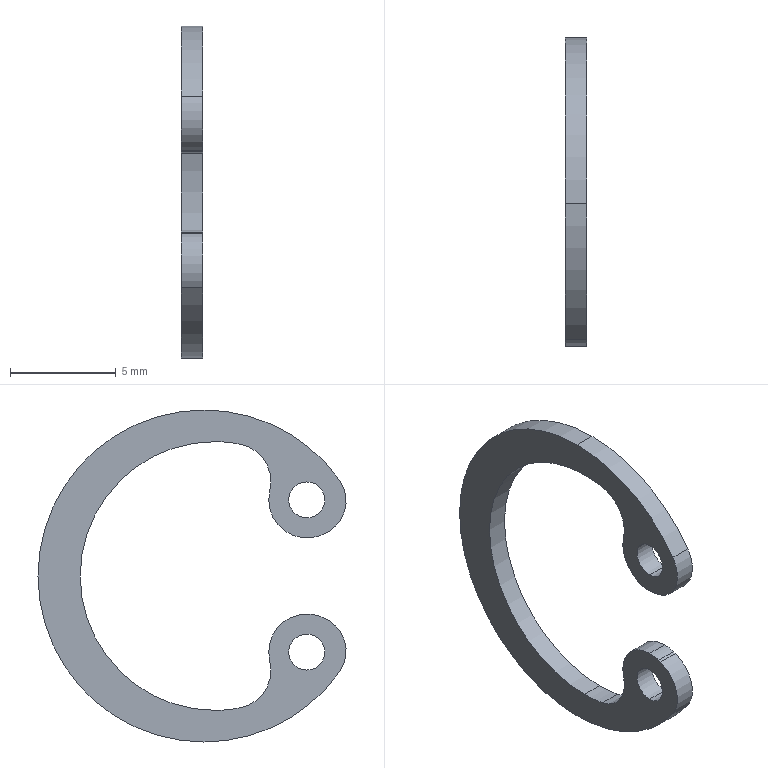Part | SolidWorks | features MBimport 1 | 1 solid | 21 faces | box 1 x 14.572 x 15.7 mm | volume 72.207 mm3 | cylinder 17 | plane 4 | commonest cylinder face diameters 3.6 x5 1.7 x4 12.7 x3 15.7 x3 3.4 x2
STEP:
#1=CARTESIAN_POINT('',(0.5,0.,-7.85));
#2=VERTEX_POINT('',#1);
#3=CARTESIAN_POINT('',(0.5,0.,7.85));
#4=VERTEX_POINT('',#3);
#5=CARTESIAN_POINT('',(0.5,0.,0.));
#6=DIRECTION('',(1.,0.,0.));
#7=DIRECTION('',(0.,0.,-1.));
#8=AXIS2_PLACEMENT_3D('',#5,#6,#7);
#9=CIRCLE('',#8,7.85);
#10=EDGE_CURVE('',#2,#4,#9,.T.);
#11=ORIENTED_EDGE('',*,*,#10,.F.);
#12=CARTESIAN_POINT('',(-0.5,0.,-7.85));
#13=VERTEX_POINT('',#12);
#14=CARTESIAN_POINT('',(0.5,0.,-7.85));
#15=DIRECTION('',(-1.,0.,0.));
#16=VECTOR('',#15,1000.);
#17=LINE('',#14,#16);
#18=EDGE_CURVE('',#2,#13,#17,.T.);
#19=ORIENTED_EDGE('',*,*,#18,.T.);
#20=CARTESIAN_POINT('',(-0.5,0.,7.85));
#21=VERTEX_POINT('',#20);
#22=CARTESIAN_POINT('',(-0.5,0.,0.));
#23=DIRECTION('',(1.,0.,0.));
#24=DIRECTION('',(0.,0.,-1.));
#25=AXIS2_PLACEMENT_3D('',#22,#23,#24);
#26=CIRCLE('',#25,7.85);
#27=EDGE_CURVE('',#13,#21,#26,.T.);
#28=ORIENTED_EDGE('',*,*,#27,.T.);
#29=CARTESIAN_POINT('',(0.5,0.,7.85));
#30=DIRECTION('',(-1.,0.,0.));
#31=VECTOR('',#30,1000.);
#32=LINE('',#29,#31);
#33=EDGE_CURVE('',#4,#21,#32,.T.);
#34=ORIENTED_EDGE('',*,*,#33,.F.);
#35=EDGE_LOOP('',(#11,#19,#28,#34));
#36=FACE_OUTER_BOUND('',#35,.T.);
#37=CARTESIAN_POINT('',(0.5,0.,0.));
#38=DIRECTION('',(-1.,0.,0.));
#39=DIRECTION('',(0.,0.,1.));
#40=AXIS2_PLACEMENT_3D('',#37,#38,#39);
#41=CYLINDRICAL_SURFACE('',#40,7.85);
#42=ADVANCED_FACE('',(#36),#41,.T.);
#43=CARTESIAN_POINT('',(0.5,-6.41,4.531));
#44=VERTEX_POINT('',#43);
#45=CARTESIAN_POINT('',(0.5,0.,0.));
#46=DIRECTION('',(1.,0.,0.));
#47=DIRECTION('',(0.,0.,-1.));
#48=AXIS2_PLACEMENT_3D('',#45,#46,#47);
#49=CIRCLE('',#48,7.85);
#50=EDGE_CURVE('',#4,#44,#49,.T.);
#51=ORIENTED_EDGE('',*,*,#50,.F.);
#52=ORIENTED_EDGE('',*,*,#33,.T.);
#53=CARTESIAN_POINT('',(-0.5,-6.41,4.531));
#54=VERTEX_POINT('',#53);
#55=CARTESIAN_POINT('',(-0.5,0.,0.));
#56=DIRECTION('',(1.,0.,0.));
#57=DIRECTION('',(0.,0.,-1.));
#58=AXIS2_PLACEMENT_3D('',#55,#56,#57);
#59=CIRCLE('',#58,7.85);
#60=EDGE_CURVE('',#21,#54,#59,.T.);
#61=ORIENTED_EDGE('',*,*,#60,.T.);
#62=CARTESIAN_POINT('',(0.5,-6.41,4.531));
#63=DIRECTION('',(-1.,0.,0.));
#64=VECTOR('',#63,1000.);
#65=LINE('',#62,#64);
#66=EDGE_CURVE('',#44,#54,#65,.T.);
#67=ORIENTED_EDGE('',*,*,#66,.F.);
#68=EDGE_LOOP('',(#51,#52,#61,#67));
#69=FACE_OUTER_BOUND('',#68,.T.);
#70=CARTESIAN_POINT('',(0.5,0.,0.));
#71=DIRECTION('',(-1.,0.,0.));
#72=DIRECTION('',(0.,0.,1.));
#73=AXIS2_PLACEMENT_3D('',#70,#71,#72);
#74=CYLINDRICAL_SURFACE('',#73,7.85);
#75=ADVANCED_FACE('',(#69),#74,.T.);
#76=CARTESIAN_POINT('',(0.5,-1.712,-6.233));
#77=VERTEX_POINT('',#76);
#78=CARTESIAN_POINT('',(0.5,-0.5,-6.35));
#79=VERTEX_POINT('',#78);
#80=CARTESIAN_POINT('',(0.5,-0.5,0.));
#81=DIRECTION('',(1.,0.,0.));
#82=DIRECTION('',(0.,0.,-1.));
#83=AXIS2_PLACEMENT_3D('',#80,#81,#82);
#84=CIRCLE('',#83,6.35);
#85=EDGE_CURVE('',#77,#79,#84,.T.);
#86=ORIENTED_EDGE('',*,*,#85,.T.);
#87=CARTESIAN_POINT('',(-0.5,-0.5,-6.35));
#88=VERTEX_POINT('',#87);
#89=CARTESIAN_POINT('',(0.5,-0.5,-6.35));
#90=DIRECTION('',(-1.,0.,0.));
#91=VECTOR('',#90,1000.);
#92=LINE('',#89,#91);
#93=EDGE_CURVE('',#79,#88,#92,.T.);
#94=ORIENTED_EDGE('',*,*,#93,.T.);
#95=CARTESIAN_POINT('',(-0.5,-1.712,-6.233));
#96=VERTEX_POINT('',#95);
#97=CARTESIAN_POINT('',(-0.5,-0.5,0.));
#98=DIRECTION('',(1.,0.,0.));
#99=DIRECTION('',(0.,0.,-1.));
#100=AXIS2_PLACEMENT_3D('',#97,#98,#99);
#101=CIRCLE('',#100,6.35);
#102=EDGE_CURVE('',#96,#88,#101,.T.);
#103=ORIENTED_EDGE('',*,*,#102,.F.);
#104=CARTESIAN_POINT('',(0.5,-1.712,-6.233));
#105=DIRECTION('',(-1.,0.,0.));
#106=VECTOR('',#105,1000.);
#107=LINE('',#104,#106);
#108=EDGE_CURVE('',#77,#96,#107,.T.);
#109=ORIENTED_EDGE('',*,*,#108,.F.);
#110=EDGE_LOOP('',(#86,#94,#103,#109));
#111=FACE_OUTER_BOUND('',#110,.T.);
#112=CARTESIAN_POINT('',(0.5,-0.5,0.));
#113=DIRECTION('',(-1.,0.,0.));
#114=DIRECTION('',(0.,0.,1.));
#115=AXIS2_PLACEMENT_3D('',#112,#113,#114);
#116=CYLINDRICAL_SURFACE('',#115,6.35);
#117=ADVANCED_FACE('',(#111),#116,.F.);
#118=ORIENTED_EDGE('',*,*,#93,.F.);
#119=CARTESIAN_POINT('',(0.5,-0.5,6.35));
#120=VERTEX_POINT('',#119);
#121=CARTESIAN_POINT('',(0.5,-0.5,0.));
#122=DIRECTION('',(1.,0.,0.));
#123=DIRECTION('',(0.,0.,-1.));
#124=AXIS2_PLACEMENT_3D('',#121,#122,#123);
#125=CIRCLE('',#124,6.35);
#126=EDGE_CURVE('',#79,#120,#125,.T.);
#127=ORIENTED_EDGE('',*,*,#126,.T.);
#128=CARTESIAN_POINT('',(-0.5,-0.5,6.35));
#129=VERTEX_POINT('',#128);
#130=CARTESIAN_POINT('',(0.5,-0.5,6.35));
#131=DIRECTION('',(-1.,0.,0.));
#132=VECTOR('',#131,1000.);
#133=LINE('',#130,#132);
#134=EDGE_CURVE('',#120,#129,#133,.T.);
#135=ORIENTED_EDGE('',*,*,#134,.T.);
#136=CARTESIAN_POINT('',(-0.5,-0.5,0.));
#137=DIRECTION('',(1.,0.,0.));
#138=DIRECTION('',(0.,0.,-1.));
#139=AXIS2_PLACEMENT_3D('',#136,#137,#138);
#140=CIRCLE('',#139,6.35);
#141=EDGE_CURVE('',#88,#129,#140,.T.);
#142=ORIENTED_EDGE('',*,*,#141,.F.);
#143=EDGE_LOOP('',(#118,#127,#135,#142));
#144=FACE_OUTER_BOUND('',#143,.T.);
#145=CARTESIAN_POINT('',(0.5,-0.5,0.));
#146=DIRECTION('',(-1.,0.,0.));
#147=DIRECTION('',(0.,0.,1.));
#148=AXIS2_PLACEMENT_3D('',#145,#146,#147);
#149=CYLINDRICAL_SURFACE('',#148,6.35);
#150=ADVANCED_FACE('',(#144),#149,.F.);
#151=CARTESIAN_POINT('',(0.5,-4.862,-1.8));
#152=VERTEX_POINT('',#151);
#153=CARTESIAN_POINT('',(0.5,-5.455,-1.9));
#154=VERTEX_POINT('',#153);
#155=CARTESIAN_POINT('',(0.5,-4.862,-3.6));
#156=DIRECTION('',(1.,0.,0.));
#157=DIRECTION('',(0.,0.,-1.));
#158=AXIS2_PLACEMENT_3D('',#155,#156,#157);
#159=CIRCLE('',#158,1.8);
#160=EDGE_CURVE('',#152,#154,#159,.T.);
#161=ORIENTED_EDGE('',*,*,#160,.F.);
#162=CARTESIAN_POINT('',(-0.5,-4.862,-1.8));
#163=VERTEX_POINT('',#162);
#164=CARTESIAN_POINT('',(0.5,-4.862,-1.8));
#165=DIRECTION('',(-1.,0.,0.));
#166=VECTOR('',#165,1000.);
#167=LINE('',#164,#166);
#168=EDGE_CURVE('',#152,#163,#167,.T.);
#169=ORIENTED_EDGE('',*,*,#168,.T.);
#170=CARTESIAN_POINT('',(-0.5,-5.455,-1.9));
#171=VERTEX_POINT('',#170);
#172=CARTESIAN_POINT('',(-0.5,-4.862,-3.6));
#173=DIRECTION('',(1.,0.,0.));
#174=DIRECTION('',(0.,0.,-1.));
#175=AXIS2_PLACEMENT_3D('',#172,#173,#174);
#176=CIRCLE('',#175,1.8);
#177=EDGE_CURVE('',#163,#171,#176,.T.);
#178=ORIENTED_EDGE('',*,*,#177,.T.);
#179=CARTESIAN_POINT('',(0.5,-5.455,-1.9));
#180=DIRECTION('',(-1.,0.,0.));
#181=VECTOR('',#180,1000.);
#182=LINE('',#179,#181);
#183=EDGE_CURVE('',#154,#171,#182,.T.);
#184=ORIENTED_EDGE('',*,*,#183,.F.);
#185=EDGE_LOOP('',(#161,#169,#178,#184));
#186=FACE_OUTER_BOUND('',#185,.T.);
#187=CARTESIAN_POINT('',(0.5,-4.862,-3.6));
#188=DIRECTION('',(-1.,0.,0.));
#189=DIRECTION('',(0.,0.,1.));
#190=AXIS2_PLACEMENT_3D('',#187,#188,#189);
#191=CYLINDRICAL_SURFACE('',#190,1.8);
#192=ADVANCED_FACE('',(#186),#191,.T.);
#193=CARTESIAN_POINT('',(0.5,-4.862,-2.75));
#194=VERTEX_POINT('',#193);
#195=CARTESIAN_POINT('',(0.5,-4.862,-4.45));
#196=VERTEX_POINT('',#195);
#197=CARTESIAN_POINT('',(0.5,-4.862,-3.6));
#198=DIRECTION('',(1.,0.,0.));
#199=DIRECTION('',(0.,0.,-1.));
#200=AXIS2_PLACEMENT_3D('',#197,#198,#199);
#201=CIRCLE('',#200,0.85);
#202=EDGE_CURVE('',#194,#196,#201,.T.);
#203=ORIENTED_EDGE('',*,*,#202,.T.);
#204=CARTESIAN_POINT('',(-0.5,-4.862,-4.45));
#205=VERTEX_POINT('',#204);
#206=CARTESIAN_POINT('',(0.5,-4.862,-4.45));
#207=DIRECTION('',(-1.,0.,0.));
#208=VECTOR('',#207,1000.);
#209=LINE('',#206,#208);
#210=EDGE_CURVE('',#196,#205,#209,.T.);
#211=ORIENTED_EDGE('',*,*,#210,.T.);
#212=CARTESIAN_POINT('',(-0.5,-4.862,-2.75));
#213=VERTEX_POINT('',#212);
#214=CARTESIAN_POINT('',(-0.5,-4.862,-3.6));
#215=DIRECTION('',(1.,0.,0.));
#216=DIRECTION('',(0.,0.,-1.));
#217=AXIS2_PLACEMENT_3D('',#214,#215,#216);
#218=CIRCLE('',#217,0.85);
#219=EDGE_CURVE('',#213,#205,#218,.T.);
#220=ORIENTED_EDGE('',*,*,#219,.F.);
#221=CARTESIAN_POINT('',(0.5,-4.862,-2.75));
#222=DIRECTION('',(-1.,0.,0.));
#223=VECTOR('',#222,1000.);
#224=LINE('',#221,#223);
#225=EDGE_CURVE('',#194,#213,#224,.T.);
#226=ORIENTED_EDGE('',*,*,#225,.F.);
#227=EDGE_LOOP('',(#203,#211,#220,#226));
#228=FACE_OUTER_BOUND('',#227,.T.);
#229=CARTESIAN_POINT('',(0.5,-4.862,-3.6));
#230=DIRECTION('',(-1.,0.,0.));
#231=DIRECTION('',(0.,0.,1.));
#232=AXIS2_PLACEMENT_3D('',#229,#230,#231);
#233=CYLINDRICAL_SURFACE('',#232,0.85);
#234=ADVANCED_FACE('',(#228),#233,.F.);
#235=CARTESIAN_POINT('',(0.5,-4.862,4.45));
#236=VERTEX_POINT('',#235);
#237=CARTESIAN_POINT('',(0.5,-4.862,2.75));
#238=VERTEX_POINT('',#237);
#239=CARTESIAN_POINT('',(0.5,-4.862,3.6));
#240=DIRECTION('',(1.,0.,0.));
#241=DIRECTION('',(0.,0.,-1.));
#242=AXIS2_PLACEMENT_3D('',#239,#240,#241);
#243=CIRCLE('',#242,0.85);
#244=EDGE_CURVE('',#236,#238,#243,.T.);
#245=ORIENTED_EDGE('',*,*,#244,.T.);
#246=CARTESIAN_POINT('',(-0.5,-4.862,2.75));
#247=VERTEX_POINT('',#246);
#248=CARTESIAN_POINT('',(0.5,-4.862,2.75));
#249=DIRECTION('',(-1.,0.,0.));
#250=VECTOR('',#249,1000.);
#251=LINE('',#248,#250);
#252=EDGE_CURVE('',#238,#247,#251,.T.);
#253=ORIENTED_EDGE('',*,*,#252,.T.);
#254=CARTESIAN_POINT('',(-0.5,-4.862,4.45));
#255=VERTEX_POINT('',#254);
#256=CARTESIAN_POINT('',(-0.5,-4.862,3.6));
#257=DIRECTION('',(1.,0.,0.));
#258=DIRECTION('',(0.,0.,-1.));
#259=AXIS2_PLACEMENT_3D('',#256,#257,#258);
#260=CIRCLE('',#259,0.85);
#261=EDGE_CURVE('',#255,#247,#260,.T.);
#262=ORIENTED_EDGE('',*,*,#261,.F.);
#263=CARTESIAN_POINT('',(0.5,-4.862,4.45));
#264=DIRECTION('',(-1.,0.,0.));
#265=VECTOR('',#264,1000.);
#266=LINE('',#263,#265);
#267=EDGE_CURVE('',#236,#255,#266,.T.);
#268=ORIENTED_EDGE('',*,*,#267,.F.);
#269=EDGE_LOOP('',(#245,#253,#262,#268));
#270=FACE_OUTER_BOUND('',#269,.T.);
#271=CARTESIAN_POINT('',(0.5,-4.862,3.6));
#272=DIRECTION('',(-1.,0.,0.));
#273=DIRECTION('',(0.,0.,1.));
#274=AXIS2_PLACEMENT_3D('',#271,#272,#273);
#275=CYLINDRICAL_SURFACE('',#274,0.85);
#276=ADVANCED_FACE('',(#270),#275,.F.);
#277=CARTESIAN_POINT('',(-0.5,-5.581,-1.944));
#278=VERTEX_POINT('',#277);
#279=CARTESIAN_POINT('',(-0.5,-6.41,-4.531));
#280=VERTEX_POINT('',#279);
#281=CARTESIAN_POINT('',(-0.5,-5.022,-3.55));
#282=DIRECTION('',(1.,0.,0.));
#283=DIRECTION('',(0.,0.,-1.));
#284=AXIS2_PLACEMENT_3D('',#281,#282,#283);
#285=CIRCLE('',#284,1.7);
#286=EDGE_CURVE('',#278,#280,#285,.T.);
#287=ORIENTED_EDGE('',*,*,#286,.F.);
#288=CARTESIAN_POINT('',(-0.5,-5.455,-1.9));
#289=DIRECTION('',(0.,-0.9443,-0.329));
#290=VECTOR('',#289,1000.);
#291=LINE('',#288,#290);
#292=EDGE_CURVE('',#171,#278,#291,.T.);
#293=ORIENTED_EDGE('',*,*,#292,.F.);
#294=ORIENTED_EDGE('',*,*,#177,.F.);
#295=CARTESIAN_POINT('',(-0.5,-3.115,-4.033));
#296=VERTEX_POINT('',#295);
#297=CARTESIAN_POINT('',(-0.5,-4.862,-3.6));
#298=DIRECTION('',(1.,0.,0.));
#299=DIRECTION('',(0.,0.,-1.));
#300=AXIS2_PLACEMENT_3D('',#297,#298,#299);
#301=CIRCLE('',#300,1.8);
#302=EDGE_CURVE('',#296,#163,#301,.T.);
#303=ORIENTED_EDGE('',*,*,#302,.F.);
#304=CARTESIAN_POINT('',(-0.5,-1.368,-4.466));
#305=DIRECTION('',(1.,0.,0.));
#306=DIRECTION('',(0.,0.,-1.));
#307=AXIS2_PLACEMENT_3D('',#304,#305,#306);
#308=CIRCLE('',#307,1.8);
#309=EDGE_CURVE('',#296,#96,#308,.T.);
#310=ORIENTED_EDGE('',*,*,#309,.T.);
#311=ORIENTED_EDGE('',*,*,#102,.T.);
#312=ORIENTED_EDGE('',*,*,#141,.T.);
#313=CARTESIAN_POINT('',(-0.5,-1.712,6.233));
#314=VERTEX_POINT('',#313);
#315=CARTESIAN_POINT('',(-0.5,-0.5,0.));
#316=DIRECTION('',(1.,0.,0.));
#317=DIRECTION('',(0.,0.,-1.));
#318=AXIS2_PLACEMENT_3D('',#315,#316,#317);
#319=CIRCLE('',#318,6.35);
#320=EDGE_CURVE('',#129,#314,#319,.T.);
#321=ORIENTED_EDGE('',*,*,#320,.T.);
#322=CARTESIAN_POINT('',(-0.5,-3.115,4.033));
#323=VERTEX_POINT('',#322);
#324=CARTESIAN_POINT('',(-0.5,-1.368,4.466));
#325=DIRECTION('',(1.,0.,0.));
#326=DIRECTION('',(0.,0.,-1.));
#327=AXIS2_PLACEMENT_3D('',#324,#325,#326);
#328=CIRCLE('',#327,1.8);
#329=EDGE_CURVE('',#314,#323,#328,.T.);
#330=ORIENTED_EDGE('',*,*,#329,.T.);
#331=CARTESIAN_POINT('',(-0.5,-5.455,1.9));
#332=VERTEX_POINT('',#331);
#333=CARTESIAN_POINT('',(-0.5,-4.862,3.6));
#334=DIRECTION('',(1.,0.,0.));
#335=DIRECTION('',(0.,0.,-1.));
#336=AXIS2_PLACEMENT_3D('',#333,#334,#335);
#337=CIRCLE('',#336,1.8);
#338=EDGE_CURVE('',#332,#323,#337,.T.);
#339=ORIENTED_EDGE('',*,*,#338,.F.);
#340=CARTESIAN_POINT('',(-0.5,-5.581,1.944));
#341=VERTEX_POINT('',#340);
#342=CARTESIAN_POINT('',(-0.5,-5.581,1.944));
#343=DIRECTION('',(0.,0.9443,-0.329));
#344=VECTOR('',#343,1000.);
#345=LINE('',#342,#344);
#346=EDGE_CURVE('',#341,#332,#345,.T.);
#347=ORIENTED_EDGE('',*,*,#346,.F.);
#348=CARTESIAN_POINT('',(-0.5,-5.022,3.55));
#349=DIRECTION('',(1.,0.,0.));
#350=DIRECTION('',(0.,0.,-1.));
#351=AXIS2_PLACEMENT_3D('',#348,#349,#350);
#352=CIRCLE('',#351,1.7);
#353=EDGE_CURVE('',#54,#341,#352,.T.);
#354=ORIENTED_EDGE('',*,*,#353,.F.);
#355=ORIENTED_EDGE('',*,*,#60,.F.);
#356=ORIENTED_EDGE('',*,*,#27,.F.);
#357=CARTESIAN_POINT('',(-0.5,0.,0.));
#358=DIRECTION('',(1.,0.,0.));
#359=DIRECTION('',(0.,0.,-1.));
#360=AXIS2_PLACEMENT_3D('',#357,#358,#359);
#361=CIRCLE('',#360,7.85);
#362=EDGE_CURVE('',#280,#13,#361,.T.);
#363=ORIENTED_EDGE('',*,*,#362,.F.);
#364=EDGE_LOOP('',(#287,#293,#294,#303,#310,#311,#312,#321,#330,#339,#347,#354,#355,#356,#363));
#365=FACE_OUTER_BOUND('',#364,.T.);
#366=ORIENTED_EDGE('',*,*,#219,.T.);
#367=CARTESIAN_POINT('',(-0.5,-4.862,-3.6));
#368=DIRECTION('',(1.,0.,0.));
#369=DIRECTION('',(0.,0.,-1.));
#370=AXIS2_PLACEMENT_3D('',#367,#368,#369);
#371=CIRCLE('',#370,0.85);
#372=EDGE_CURVE('',#205,#213,#371,.T.);
#373=ORIENTED_EDGE('',*,*,#372,.T.);
#374=EDGE_LOOP('',(#366,#373));
#375=FACE_BOUND('',#374,.T.);
#376=ORIENTED_EDGE('',*,*,#261,.T.);
#377=CARTESIAN_POINT('',(-0.5,-4.862,3.6));
#378=DIRECTION('',(1.,0.,0.));
#379=DIRECTION('',(0.,0.,-1.));
#380=AXIS2_PLACEMENT_3D('',#377,#378,#379);
#381=CIRCLE('',#380,0.85);
#382=EDGE_CURVE('',#247,#255,#381,.T.);
#383=ORIENTED_EDGE('',*,*,#382,.T.);
#384=EDGE_LOOP('',(#376,#383));
#385=FACE_BOUND('',#384,.T.);
#386=CARTESIAN_POINT('',(-0.5,-5.022,-3.55));
#387=DIRECTION('',(1.,0.,0.));
#388=DIRECTION('',(0.,1.,0.));
#389=AXIS2_PLACEMENT_3D('',#386,#387,#388);
#390=PLANE('',#389);
#391=ADVANCED_FACE('',(#365,#375,#385),#390,.F.);
#392=CARTESIAN_POINT('',(0.5,-5.581,-1.944));
#393=VERTEX_POINT('',#392);
#394=CARTESIAN_POINT('',(0.5,-6.41,-4.531));
#395=VERTEX_POINT('',#394);
#396=CARTESIAN_POINT('',(0.5,-5.022,-3.55));
#397=DIRECTION('',(1.,0.,0.));
#398=DIRECTION('',(0.,0.,-1.));
#399=AXIS2_PLACEMENT_3D('',#396,#397,#398);
#400=CIRCLE('',#399,1.7);
#401=EDGE_CURVE('',#393,#395,#400,.T.);
#402=ORIENTED_EDGE('',*,*,#401,.T.);
#403=CARTESIAN_POINT('',(0.5,0.,0.));
#404=DIRECTION('',(1.,0.,0.));
#405=DIRECTION('',(0.,0.,-1.));
#406=AXIS2_PLACEMENT_3D('',#403,#404,#405);
#407=CIRCLE('',#406,7.85);
#408=EDGE_CURVE('',#395,#2,#407,.T.);
#409=ORIENTED_EDGE('',*,*,#408,.T.);
#410=ORIENTED_EDGE('',*,*,#10,.T.);
#411=ORIENTED_EDGE('',*,*,#50,.T.);
#412=CARTESIAN_POINT('',(0.5,-5.581,1.944));
#413=VERTEX_POINT('',#412);
#414=CARTESIAN_POINT('',(0.5,-5.022,3.55));
#415=DIRECTION('',(1.,0.,0.));
#416=DIRECTION('',(0.,0.,-1.));
#417=AXIS2_PLACEMENT_3D('',#414,#415,#416);
#418=CIRCLE('',#417,1.7);
#419=EDGE_CURVE('',#44,#413,#418,.T.);
#420=ORIENTED_EDGE('',*,*,#419,.T.);
#421=CARTESIAN_POINT('',(0.5,-5.455,1.9));
#422=VERTEX_POINT('',#421);
#423=CARTESIAN_POINT('',(0.5,-5.581,1.944));
#424=DIRECTION('',(0.,0.9443,-0.329));
#425=VECTOR('',#424,1000.);
#426=LINE('',#423,#425);
#427=EDGE_CURVE('',#413,#422,#426,.T.);
#428=ORIENTED_EDGE('',*,*,#427,.T.);
#429=CARTESIAN_POINT('',(0.5,-3.115,4.033));
#430=VERTEX_POINT('',#429);
#431=CARTESIAN_POINT('',(0.5,-4.862,3.6));
#432=DIRECTION('',(1.,0.,0.));
#433=DIRECTION('',(0.,0.,-1.));
#434=AXIS2_PLACEMENT_3D('',#431,#432,#433);
#435=CIRCLE('',#434,1.8);
#436=EDGE_CURVE('',#422,#430,#435,.T.);
#437=ORIENTED_EDGE('',*,*,#436,.T.);
#438=CARTESIAN_POINT('',(0.5,-1.712,6.233));
#439=VERTEX_POINT('',#438);
#440=CARTESIAN_POINT('',(0.5,-1.368,4.466));
#441=DIRECTION('',(1.,0.,0.));
#442=DIRECTION('',(0.,0.,-1.));
#443=AXIS2_PLACEMENT_3D('',#440,#441,#442);
#444=CIRCLE('',#443,1.8);
#445=EDGE_CURVE('',#439,#430,#444,.T.);
#446=ORIENTED_EDGE('',*,*,#445,.F.);
#447=CARTESIAN_POINT('',(0.5,-0.5,0.));
#448=DIRECTION('',(1.,0.,0.));
#449=DIRECTION('',(0.,0.,-1.));
#450=AXIS2_PLACEMENT_3D('',#447,#448,#449);
#451=CIRCLE('',#450,6.35);
#452=EDGE_CURVE('',#120,#439,#451,.T.);
#453=ORIENTED_EDGE('',*,*,#452,.F.);
#454=ORIENTED_EDGE('',*,*,#126,.F.);
#455=ORIENTED_EDGE('',*,*,#85,.F.);
#456=CARTESIAN_POINT('',(0.5,-3.115,-4.033));
#457=VERTEX_POINT('',#456);
#458=CARTESIAN_POINT('',(0.5,-1.368,-4.466));
#459=DIRECTION('',(1.,0.,0.));
#460=DIRECTION('',(0.,0.,-1.));
#461=AXIS2_PLACEMENT_3D('',#458,#459,#460);
#462=CIRCLE('',#461,1.8);
#463=EDGE_CURVE('',#457,#77,#462,.T.);
#464=ORIENTED_EDGE('',*,*,#463,.F.);
#465=CARTESIAN_POINT('',(0.5,-4.862,-3.6));
#466=DIRECTION('',(1.,0.,0.));
#467=DIRECTION('',(0.,0.,-1.));
#468=AXIS2_PLACEMENT_3D('',#465,#466,#467);
#469=CIRCLE('',#468,1.8);
#470=EDGE_CURVE('',#457,#152,#469,.T.);
#471=ORIENTED_EDGE('',*,*,#470,.T.);
#472=ORIENTED_EDGE('',*,*,#160,.T.);
#473=CARTESIAN_POINT('',(0.5,-5.455,-1.9));
#474=DIRECTION('',(0.,-0.9443,-0.329));
#475=VECTOR('',#474,1000.);
#476=LINE('',#473,#475);
#477=EDGE_CURVE('',#154,#393,#476,.T.);
#478=ORIENTED_EDGE('',*,*,#477,.T.);
#479=EDGE_LOOP('',(#402,#409,#410,#411,#420,#428,#437,#446,#453,#454,#455,#464,#471,#472,#478));
#480=FACE_OUTER_BOUND('',#479,.T.);
#481=ORIENTED_EDGE('',*,*,#202,.F.);
#482=CARTESIAN_POINT('',(0.5,-4.862,-3.6));
#483=DIRECTION('',(1.,0.,0.));
#484=DIRECTION('',(0.,0.,-1.));
#485=AXIS2_PLACEMENT_3D('',#482,#483,#484);
#486=CIRCLE('',#485,0.85);
#487=EDGE_CURVE('',#196,#194,#486,.T.);
#488=ORIENTED_EDGE('',*,*,#487,.F.);
#489=EDGE_LOOP('',(#481,#488));
#490=FACE_BOUND('',#489,.T.);
#491=ORIENTED_EDGE('',*,*,#244,.F.);
#492=CARTESIAN_POINT('',(0.5,-4.862,3.6));
#493=DIRECTION('',(1.,0.,0.));
#494=DIRECTION('',(0.,0.,-1.));
#495=AXIS2_PLACEMENT_3D('',#492,#493,#494);
#496=CIRCLE('',#495,0.85);
#497=EDGE_CURVE('',#238,#236,#496,.T.);
#498=ORIENTED_EDGE('',*,*,#497,.F.);
#499=EDGE_LOOP('',(#491,#498));
#500=FACE_BOUND('',#499,.T.);
#501=CARTESIAN_POINT('',(0.5,-5.022,-3.55));
#502=DIRECTION('',(1.,0.,0.));
#503=DIRECTION('',(0.,1.,0.));
#504=AXIS2_PLACEMENT_3D('',#501,#502,#503);
#505=PLANE('',#504);
#506=ADVANCED_FACE('',(#480,#490,#500),#505,.T.);
#507=ORIENTED_EDGE('',*,*,#292,.T.);
#508=CARTESIAN_POINT('',(0.5,-5.581,-1.944));
#509=DIRECTION('',(-1.,0.,0.));
#510=VECTOR('',#509,1000.);
#511=LINE('',#508,#510);
#512=EDGE_CURVE('',#393,#278,#511,.T.);
#513=ORIENTED_EDGE('',*,*,#512,.F.);
#514=ORIENTED_EDGE('',*,*,#477,.F.);
#515=ORIENTED_EDGE('',*,*,#183,.T.);
#516=EDGE_LOOP('',(#507,#513,#514,#515));
#517=FACE_OUTER_BOUND('',#516,.T.);
#518=CARTESIAN_POINT('',(0.5,-5.455,-1.9));
#519=DIRECTION('',(0.,0.329,-0.9443));
#520=DIRECTION('',(-1.,0.,0.));
#521=AXIS2_PLACEMENT_3D('',#518,#519,#520);
#522=PLANE('',#521);
#523=ADVANCED_FACE('',(#517),#522,.F.);
#524=ORIENTED_EDGE('',*,*,#252,.F.);
#525=ORIENTED_EDGE('',*,*,#497,.T.);
#526=ORIENTED_EDGE('',*,*,#267,.T.);
#527=ORIENTED_EDGE('',*,*,#382,.F.);
#528=EDGE_LOOP('',(#524,#525,#526,#527));
#529=FACE_OUTER_BOUND('',#528,.T.);
#530=CARTESIAN_POINT('',(0.5,-4.862,3.6));
#531=DIRECTION('',(-1.,0.,0.));
#532=DIRECTION('',(0.,0.,1.));
#533=AXIS2_PLACEMENT_3D('',#530,#531,#532);
#534=CYLINDRICAL_SURFACE('',#533,0.85);
#535=ADVANCED_FACE('',(#529),#534,.F.);
#536=ORIENTED_EDGE('',*,*,#210,.F.);
#537=ORIENTED_EDGE('',*,*,#487,.T.);
#538=ORIENTED_EDGE('',*,*,#225,.T.);
#539=ORIENTED_EDGE('',*,*,#372,.F.);
#540=EDGE_LOOP('',(#536,#537,#538,#539));
#541=FACE_OUTER_BOUND('',#540,.T.);
#542=CARTESIAN_POINT('',(0.5,-4.862,-3.6));
#543=DIRECTION('',(-1.,0.,0.));
#544=DIRECTION('',(0.,0.,1.));
#545=AXIS2_PLACEMENT_3D('',#542,#543,#544);
#546=CYLINDRICAL_SURFACE('',#545,0.85);
#547=ADVANCED_FACE('',(#541),#546,.F.);
#548=ORIENTED_EDGE('',*,*,#168,.F.);
#549=ORIENTED_EDGE('',*,*,#470,.F.);
#550=CARTESIAN_POINT('',(0.5,-3.115,-4.033));
#551=DIRECTION('',(-1.,0.,0.));
#552=VECTOR('',#551,1000.);
#553=LINE('',#550,#552);
#554=EDGE_CURVE('',#457,#296,#553,.T.);
#555=ORIENTED_EDGE('',*,*,#554,.T.);
#556=ORIENTED_EDGE('',*,*,#302,.T.);
#557=EDGE_LOOP('',(#548,#549,#555,#556));
#558=FACE_OUTER_BOUND('',#557,.T.);
#559=CARTESIAN_POINT('',(0.5,-4.862,-3.6));
#560=DIRECTION('',(-1.,0.,0.));
#561=DIRECTION('',(0.,0.,1.));
#562=AXIS2_PLACEMENT_3D('',#559,#560,#561);
#563=CYLINDRICAL_SURFACE('',#562,1.8);
#564=ADVANCED_FACE('',(#558),#563,.T.);
#565=ORIENTED_EDGE('',*,*,#309,.F.);
#566=ORIENTED_EDGE('',*,*,#554,.F.);
#567=ORIENTED_EDGE('',*,*,#463,.T.);
#568=ORIENTED_EDGE('',*,*,#108,.T.);
#569=EDGE_LOOP('',(#565,#566,#567,#568));
#570=FACE_OUTER_BOUND('',#569,.T.);
#571=CARTESIAN_POINT('',(0.5,-1.368,-4.466));
#572=DIRECTION('',(-1.,0.,0.));
#573=DIRECTION('',(0.,0.,1.));
#574=AXIS2_PLACEMENT_3D('',#571,#572,#573);
#575=CYLINDRICAL_SURFACE('',#574,1.8);
#576=ADVANCED_FACE('',(#570),#575,.F.);
#577=ORIENTED_EDGE('',*,*,#134,.F.);
#578=ORIENTED_EDGE('',*,*,#452,.T.);
#579=CARTESIAN_POINT('',(0.5,-1.712,6.233));
#580=DIRECTION('',(-1.,0.,0.));
#581=VECTOR('',#580,1000.);
#582=LINE('',#579,#581);
#583=EDGE_CURVE('',#439,#314,#582,.T.);
#584=ORIENTED_EDGE('',*,*,#583,.T.);
#585=ORIENTED_EDGE('',*,*,#320,.F.);
#586=EDGE_LOOP('',(#577,#578,#584,#585));
#587=FACE_OUTER_BOUND('',#586,.T.);
#588=CARTESIAN_POINT('',(0.5,-0.5,0.));
#589=DIRECTION('',(-1.,0.,0.));
#590=DIRECTION('',(0.,0.,1.));
#591=AXIS2_PLACEMENT_3D('',#588,#589,#590);
#592=CYLINDRICAL_SURFACE('',#591,6.35);
#593=ADVANCED_FACE('',(#587),#592,.F.);
#594=ORIENTED_EDGE('',*,*,#329,.F.);
#595=ORIENTED_EDGE('',*,*,#583,.F.);
#596=ORIENTED_EDGE('',*,*,#445,.T.);
#597=CARTESIAN_POINT('',(0.5,-3.115,4.033));
#598=DIRECTION('',(-1.,0.,0.));
#599=VECTOR('',#598,1000.);
#600=LINE('',#597,#599);
#601=EDGE_CURVE('',#430,#323,#600,.T.);
#602=ORIENTED_EDGE('',*,*,#601,.T.);
#603=EDGE_LOOP('',(#594,#595,#596,#602));
#604=FACE_OUTER_BOUND('',#603,.T.);
#605=CARTESIAN_POINT('',(0.5,-1.368,4.466));
#606=DIRECTION('',(-1.,0.,0.));
#607=DIRECTION('',(0.,0.,1.));
#608=AXIS2_PLACEMENT_3D('',#605,#606,#607);
#609=CYLINDRICAL_SURFACE('',#608,1.8);
#610=ADVANCED_FACE('',(#604),#609,.F.);
#611=ORIENTED_EDGE('',*,*,#338,.T.);
#612=ORIENTED_EDGE('',*,*,#601,.F.);
#613=ORIENTED_EDGE('',*,*,#436,.F.);
#614=CARTESIAN_POINT('',(0.5,-5.455,1.9));
#615=DIRECTION('',(-1.,0.,0.));
#616=VECTOR('',#615,1000.);
#617=LINE('',#614,#616);
#618=EDGE_CURVE('',#422,#332,#617,.T.);
#619=ORIENTED_EDGE('',*,*,#618,.T.);
#620=EDGE_LOOP('',(#611,#612,#613,#619));
#621=FACE_OUTER_BOUND('',#620,.T.);
#622=CARTESIAN_POINT('',(0.5,-4.862,3.6));
#623=DIRECTION('',(-1.,0.,0.));
#624=DIRECTION('',(0.,0.,1.));
#625=AXIS2_PLACEMENT_3D('',#622,#623,#624);
#626=CYLINDRICAL_SURFACE('',#625,1.8);
#627=ADVANCED_FACE('',(#621),#626,.T.);
#628=ORIENTED_EDGE('',*,*,#346,.T.);
#629=ORIENTED_EDGE('',*,*,#618,.F.);
#630=ORIENTED_EDGE('',*,*,#427,.F.);
#631=CARTESIAN_POINT('',(0.5,-5.581,1.944));
#632=DIRECTION('',(-1.,0.,0.));
#633=VECTOR('',#632,1000.);
#634=LINE('',#631,#633);
#635=EDGE_CURVE('',#413,#341,#634,.T.);
#636=ORIENTED_EDGE('',*,*,#635,.T.);
#637=EDGE_LOOP('',(#628,#629,#630,#636));
#638=FACE_OUTER_BOUND('',#637,.T.);
#639=CARTESIAN_POINT('',(0.5,-5.581,1.944));
#640=DIRECTION('',(0.,0.329,0.9443));
#641=DIRECTION('',(1.,0.,0.));
#642=AXIS2_PLACEMENT_3D('',#639,#640,#641);
#643=PLANE('',#642);
#644=ADVANCED_FACE('',(#638),#643,.F.);
#645=ORIENTED_EDGE('',*,*,#353,.T.);
#646=ORIENTED_EDGE('',*,*,#635,.F.);
#647=ORIENTED_EDGE('',*,*,#419,.F.);
#648=ORIENTED_EDGE('',*,*,#66,.T.);
#649=EDGE_LOOP('',(#645,#646,#647,#648));
#650=FACE_OUTER_BOUND('',#649,.T.);
#651=CARTESIAN_POINT('',(0.5,-5.022,3.55));
#652=DIRECTION('',(-1.,0.,0.));
#653=DIRECTION('',(0.,0.,1.));
#654=AXIS2_PLACEMENT_3D('',#651,#652,#653);
#655=CYLINDRICAL_SURFACE('',#654,1.7);
#656=ADVANCED_FACE('',(#650),#655,.T.);
#657=ORIENTED_EDGE('',*,*,#18,.F.);
#658=ORIENTED_EDGE('',*,*,#408,.F.);
#659=CARTESIAN_POINT('',(0.5,-6.41,-4.531));
#660=DIRECTION('',(-1.,0.,0.));
#661=VECTOR('',#660,1000.);
#662=LINE('',#659,#661);
#663=EDGE_CURVE('',#395,#280,#662,.T.);
#664=ORIENTED_EDGE('',*,*,#663,.T.);
#665=ORIENTED_EDGE('',*,*,#362,.T.);
#666=EDGE_LOOP('',(#657,#658,#664,#665));
#667=FACE_OUTER_BOUND('',#666,.T.);
#668=CARTESIAN_POINT('',(0.5,0.,0.));
#669=DIRECTION('',(-1.,0.,0.));
#670=DIRECTION('',(0.,0.,1.));
#671=AXIS2_PLACEMENT_3D('',#668,#669,#670);
#672=CYLINDRICAL_SURFACE('',#671,7.85);
#673=ADVANCED_FACE('',(#667),#672,.T.);
#674=ORIENTED_EDGE('',*,*,#286,.T.);
#675=ORIENTED_EDGE('',*,*,#663,.F.);
#676=ORIENTED_EDGE('',*,*,#401,.F.);
#677=ORIENTED_EDGE('',*,*,#512,.T.);
#678=EDGE_LOOP('',(#674,#675,#676,#677));
#679=FACE_OUTER_BOUND('',#678,.T.);
#680=CARTESIAN_POINT('',(0.5,-5.022,-3.55));
#681=DIRECTION('',(-1.,0.,0.));
#682=DIRECTION('',(0.,0.,1.));
#683=AXIS2_PLACEMENT_3D('',#680,#681,#682);
#684=CYLINDRICAL_SURFACE('',#683,1.7);
#685=ADVANCED_FACE('',(#679),#684,.T.);
#686=CLOSED_SHELL('',(#42,#75,#117,#150,#192,#234,#276,#391,#506,#523,#535,#547,#564,#576,#593,#610,#627,#644,#656,#673,#685));
#687=MANIFOLD_SOLID_BREP('',#686);
#688=CARTESIAN_POINT('',(0.,0.,0.));
#689=DIRECTION('',(0.,0.,1.));
#690=DIRECTION('',(1.,0.,0.));
#691=AXIS2_PLACEMENT_3D('',#688,#689,#690);
#692=(LENGTH_UNIT()NAMED_UNIT(*)SI_UNIT(.MILLI.,.METRE.));
#693=UNCERTAINTY_MEASURE_WITH_UNIT(LENGTH_MEASURE(0.00001),#692,'','');
#694=(NAMED_UNIT(*)PLANE_ANGLE_UNIT()SI_UNIT($,.RADIAN.));
#695=(NAMED_UNIT(*)SI_UNIT($,.STERADIAN.)SOLID_ANGLE_UNIT());
#696=(GEOMETRIC_REPRESENTATION_CONTEXT(3)GLOBAL_UNCERTAINTY_ASSIGNED_CONTEXT((#693))GLOBAL_UNIT_ASSIGNED_CONTEXT((#692,#694,#695))REPRESENTATION_CONTEXT('',''));
#697=ADVANCED_BREP_SHAPE_REPRESENTATION('',(#687,#691),#696);